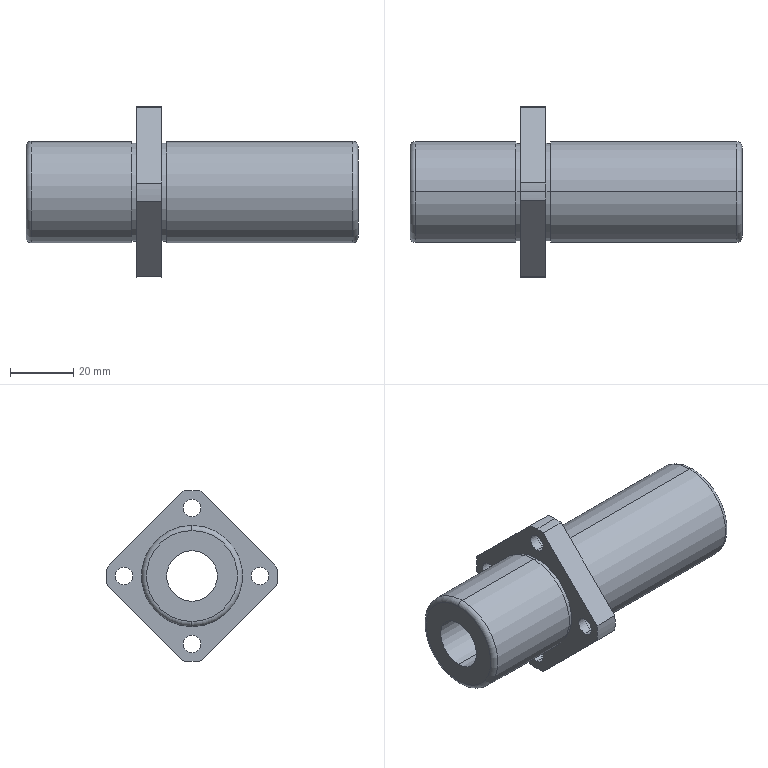Part | STEP file | LHKMSNLF16 | 1 solid | 49 faces | box 105 x 54 x 54 mm | volume 68941 mm3 | cylinder 31 | plane 14 | torus 4 | commonest cylinder face diameters 5.5 x8 9 x8 54 x5 31 x4 32 x4 16 x2